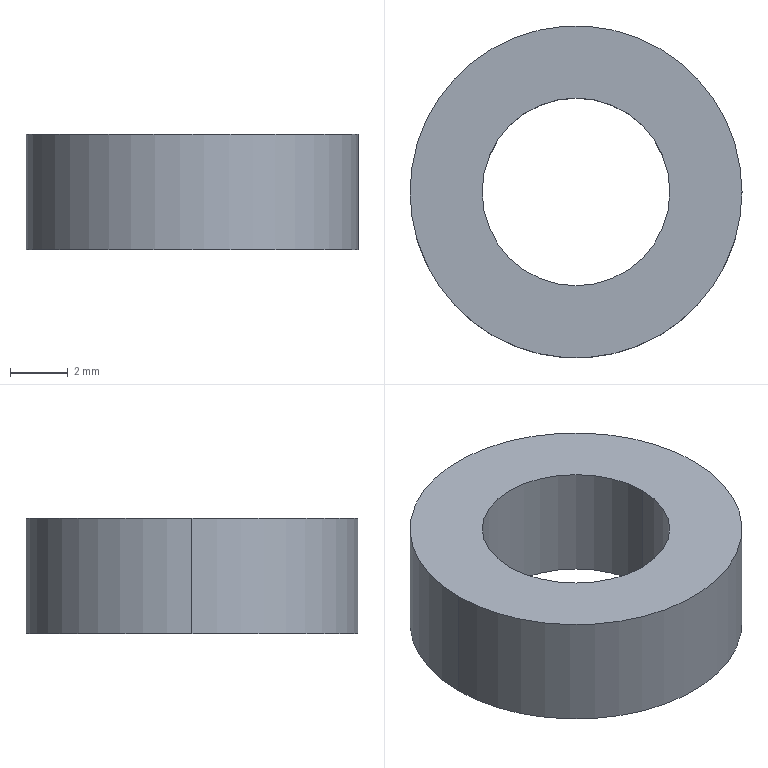Part | STEP file | Flip door spacer 001 | 1 solid | 6 faces | box 11.5 x 11.5 x 4 mm | volume 282.743 mm3 | cylinder 4 | plane 2 | commonest cylinder face diameters 6.5 x2 11.5 x2
STEP:
#1=CARTESIAN_POINT('',(0.,0.,0.));
#2=DIRECTION('',(0.,0.,1.));
#3=DIRECTION('',(1.,0.,0.));
#4=AXIS2_PLACEMENT_3D('',#1,#2,#3);
#5=CARTESIAN_POINT('',(-3.25,0.,4.));
#6=VERTEX_POINT('',#5);
#7=CARTESIAN_POINT('',(-3.25,0.,0.));
#8=VERTEX_POINT('',#7);
#9=CARTESIAN_POINT('',(-3.25,0.,4.));
#10=DIRECTION('',(0.,0.,-1.));
#11=VECTOR('',#10,1.);
#12=LINE('',#9,#11);
#13=CARTESIAN_POINT('',(0.,0.,4.));
#14=DIRECTION('',(0.,0.,-1.));
#15=DIRECTION('',(-1.,0.,0.));
#16=AXIS2_PLACEMENT_3D('',#13,#14,#15);
#17=CYLINDRICAL_SURFACE('',#16,3.25);
#18=CARTESIAN_POINT('',(6.283,0.));
#19=DIRECTION('',(0.,1.));
#20=VECTOR('',#19,1.);
#21=LINE('',#18,#20);
#22=(GEOMETRIC_REPRESENTATION_CONTEXT(2)PARAMETRIC_REPRESENTATION_CONTEXT()REPRESENTATION_CONTEXT('',''));
#23=DEFINITIONAL_REPRESENTATION('',(#21),#22);
#24=PCURVE('',#17,#23);
#25=CARTESIAN_POINT('',(0.,0.,4.));
#26=DIRECTION('',(0.,0.,-1.));
#27=DIRECTION('',(-1.,0.,0.));
#28=AXIS2_PLACEMENT_3D('',#25,#26,#27);
#29=CYLINDRICAL_SURFACE('',#28,3.25);
#30=CARTESIAN_POINT('',(0.,0.));
#31=DIRECTION('',(0.,1.));
#32=VECTOR('',#31,1.);
#33=LINE('',#30,#32);
#34=(GEOMETRIC_REPRESENTATION_CONTEXT(2)PARAMETRIC_REPRESENTATION_CONTEXT()REPRESENTATION_CONTEXT('',''));
#35=DEFINITIONAL_REPRESENTATION('',(#33),#34);
#36=PCURVE('',#29,#35);
#37=SURFACE_CURVE('',#12,(#24,#36),.PCURVE_S1.);
#38=EDGE_CURVE('',#6,#8,#37,.T.);
#39=ORIENTED_EDGE('',*,*,#38,.T.);
#40=CARTESIAN_POINT('',(3.25,0.,0.));
#41=VERTEX_POINT('',#40);
#42=CARTESIAN_POINT('',(0.,0.,0.));
#43=DIRECTION('',(0.,0.,1.));
#44=DIRECTION('',(1.,0.,0.));
#45=AXIS2_PLACEMENT_3D('',#42,#43,#44);
#46=CIRCLE('',#45,3.25);
#47=CARTESIAN_POINT('',(9.425,4.));
#48=DIRECTION('',(-1.,0.));
#49=VECTOR('',#48,1.);
#50=LINE('',#47,#49);
#51=(GEOMETRIC_REPRESENTATION_CONTEXT(2)PARAMETRIC_REPRESENTATION_CONTEXT()REPRESENTATION_CONTEXT('',''));
#52=DEFINITIONAL_REPRESENTATION('',(#50),#51);
#53=PCURVE('',#17,#52);
#54=CARTESIAN_POINT('',(0.,0.,0.));
#55=DIRECTION('',(0.,0.,1.));
#56=DIRECTION('',(1.,0.,0.));
#57=AXIS2_PLACEMENT_3D('',#54,#55,#56);
#58=PLANE('',#57);
#59=CARTESIAN_POINT('',(0.,0.));
#60=DIRECTION('',(1.,0.));
#61=AXIS2_PLACEMENT_2D('',#59,#60);
#62=CIRCLE('',#61,3.25);
#63=(GEOMETRIC_REPRESENTATION_CONTEXT(2)PARAMETRIC_REPRESENTATION_CONTEXT()REPRESENTATION_CONTEXT('',''));
#64=DEFINITIONAL_REPRESENTATION('',(#62),#63);
#65=PCURVE('',#58,#64);
#66=SURFACE_CURVE('',#46,(#53,#65),.PCURVE_S1.);
#67=EDGE_CURVE('',#8,#41,#66,.T.);
#68=ORIENTED_EDGE('',*,*,#67,.T.);
#69=CARTESIAN_POINT('',(3.25,0.,4.));
#70=VERTEX_POINT('',#69);
#71=CARTESIAN_POINT('',(3.25,0.,4.));
#72=DIRECTION('',(0.,0.,-1.));
#73=VECTOR('',#72,1.);
#74=LINE('',#71,#73);
#75=CARTESIAN_POINT('',(3.142,0.));
#76=DIRECTION('',(0.,1.));
#77=VECTOR('',#76,1.);
#78=LINE('',#75,#77);
#79=(GEOMETRIC_REPRESENTATION_CONTEXT(2)PARAMETRIC_REPRESENTATION_CONTEXT()REPRESENTATION_CONTEXT('',''));
#80=DEFINITIONAL_REPRESENTATION('',(#78),#79);
#81=PCURVE('',#17,#80);
#82=CARTESIAN_POINT('',(3.142,0.));
#83=DIRECTION('',(0.,1.));
#84=VECTOR('',#83,1.);
#85=LINE('',#82,#84);
#86=(GEOMETRIC_REPRESENTATION_CONTEXT(2)PARAMETRIC_REPRESENTATION_CONTEXT()REPRESENTATION_CONTEXT('',''));
#87=DEFINITIONAL_REPRESENTATION('',(#85),#86);
#88=PCURVE('',#29,#87);
#89=SURFACE_CURVE('',#74,(#81,#88),.PCURVE_S1.);
#90=EDGE_CURVE('',#70,#41,#89,.T.);
#91=ORIENTED_EDGE('',*,*,#90,.F.);
#92=CARTESIAN_POINT('',(0.,0.,4.));
#93=DIRECTION('',(0.,0.,1.));
#94=DIRECTION('',(1.,0.,0.));
#95=AXIS2_PLACEMENT_3D('',#92,#93,#94);
#96=CIRCLE('',#95,3.25);
#97=CARTESIAN_POINT('',(9.425,0.));
#98=DIRECTION('',(-1.,0.));
#99=VECTOR('',#98,1.);
#100=LINE('',#97,#99);
#101=(GEOMETRIC_REPRESENTATION_CONTEXT(2)PARAMETRIC_REPRESENTATION_CONTEXT()REPRESENTATION_CONTEXT('',''));
#102=DEFINITIONAL_REPRESENTATION('',(#100),#101);
#103=PCURVE('',#17,#102);
#104=CARTESIAN_POINT('',(0.,0.,4.));
#105=DIRECTION('',(0.,0.,1.));
#106=DIRECTION('',(1.,0.,0.));
#107=AXIS2_PLACEMENT_3D('',#104,#105,#106);
#108=PLANE('',#107);
#109=CARTESIAN_POINT('',(0.,0.));
#110=DIRECTION('',(1.,0.));
#111=AXIS2_PLACEMENT_2D('',#109,#110);
#112=CIRCLE('',#111,3.25);
#113=(GEOMETRIC_REPRESENTATION_CONTEXT(2)PARAMETRIC_REPRESENTATION_CONTEXT()REPRESENTATION_CONTEXT('',''));
#114=DEFINITIONAL_REPRESENTATION('',(#112),#113);
#115=PCURVE('',#108,#114);
#116=SURFACE_CURVE('',#96,(#103,#115),.PCURVE_S1.);
#117=EDGE_CURVE('',#6,#70,#116,.T.);
#118=ORIENTED_EDGE('',*,*,#117,.F.);
#119=EDGE_LOOP('',(#39,#68,#91,#118));
#120=FACE_BOUND('',#119,.F.);
#121=ADVANCED_FACE('',(#120),#17,.F.);
#122=CARTESIAN_POINT('',(5.75,0.,4.));
#123=VERTEX_POINT('',#122);
#124=CARTESIAN_POINT('',(-5.75,0.,4.));
#125=VERTEX_POINT('',#124);
#126=CARTESIAN_POINT('',(0.,0.,4.));
#127=DIRECTION('',(0.,0.,1.));
#128=DIRECTION('',(1.,0.,0.));
#129=AXIS2_PLACEMENT_3D('',#126,#127,#128);
#130=CIRCLE('',#129,5.75);
#131=CARTESIAN_POINT('',(0.,0.,4.));
#132=DIRECTION('',(0.,0.,-1.));
#133=DIRECTION('',(-1.,0.,0.));
#134=AXIS2_PLACEMENT_3D('',#131,#132,#133);
#135=CYLINDRICAL_SURFACE('',#134,5.75);
#136=CARTESIAN_POINT('',(3.142,0.));
#137=DIRECTION('',(-1.,0.));
#138=VECTOR('',#137,1.);
#139=LINE('',#136,#138);
#140=(GEOMETRIC_REPRESENTATION_CONTEXT(2)PARAMETRIC_REPRESENTATION_CONTEXT()REPRESENTATION_CONTEXT('',''));
#141=DEFINITIONAL_REPRESENTATION('',(#139),#140);
#142=PCURVE('',#135,#141);
#143=CARTESIAN_POINT('',(0.,0.));
#144=DIRECTION('',(1.,0.));
#145=AXIS2_PLACEMENT_2D('',#143,#144);
#146=CIRCLE('',#145,5.75);
#147=(GEOMETRIC_REPRESENTATION_CONTEXT(2)PARAMETRIC_REPRESENTATION_CONTEXT()REPRESENTATION_CONTEXT('',''));
#148=DEFINITIONAL_REPRESENTATION('',(#146),#147);
#149=PCURVE('',#108,#148);
#150=SURFACE_CURVE('',#130,(#142,#149),.PCURVE_S1.);
#151=EDGE_CURVE('',#123,#125,#150,.T.);
#152=ORIENTED_EDGE('',*,*,#151,.F.);
#153=CARTESIAN_POINT('',(5.75,0.,0.));
#154=VERTEX_POINT('',#153);
#155=CARTESIAN_POINT('',(5.75,0.,4.));
#156=DIRECTION('',(0.,0.,-1.));
#157=VECTOR('',#156,1.);
#158=LINE('',#155,#157);
#159=CARTESIAN_POINT('',(3.142,0.));
#160=DIRECTION('',(0.,1.));
#161=VECTOR('',#160,1.);
#162=LINE('',#159,#161);
#163=(GEOMETRIC_REPRESENTATION_CONTEXT(2)PARAMETRIC_REPRESENTATION_CONTEXT()REPRESENTATION_CONTEXT('',''));
#164=DEFINITIONAL_REPRESENTATION('',(#162),#163);
#165=PCURVE('',#135,#164);
#166=CARTESIAN_POINT('',(0.,0.,4.));
#167=DIRECTION('',(0.,0.,-1.));
#168=DIRECTION('',(-1.,0.,0.));
#169=AXIS2_PLACEMENT_3D('',#166,#167,#168);
#170=CYLINDRICAL_SURFACE('',#169,5.75);
#171=CARTESIAN_POINT('',(3.142,0.));
#172=DIRECTION('',(0.,1.));
#173=VECTOR('',#172,1.);
#174=LINE('',#171,#173);
#175=(GEOMETRIC_REPRESENTATION_CONTEXT(2)PARAMETRIC_REPRESENTATION_CONTEXT()REPRESENTATION_CONTEXT('',''));
#176=DEFINITIONAL_REPRESENTATION('',(#174),#175);
#177=PCURVE('',#170,#176);
#178=SURFACE_CURVE('',#158,(#165,#177),.PCURVE_S1.);
#179=EDGE_CURVE('',#123,#154,#178,.T.);
#180=ORIENTED_EDGE('',*,*,#179,.T.);
#181=CARTESIAN_POINT('',(-5.75,0.,0.));
#182=VERTEX_POINT('',#181);
#183=CARTESIAN_POINT('',(0.,0.,0.));
#184=DIRECTION('',(0.,0.,1.));
#185=DIRECTION('',(1.,0.,0.));
#186=AXIS2_PLACEMENT_3D('',#183,#184,#185);
#187=CIRCLE('',#186,5.75);
#188=CARTESIAN_POINT('',(3.142,4.));
#189=DIRECTION('',(-1.,0.));
#190=VECTOR('',#189,1.);
#191=LINE('',#188,#190);
#192=(GEOMETRIC_REPRESENTATION_CONTEXT(2)PARAMETRIC_REPRESENTATION_CONTEXT()REPRESENTATION_CONTEXT('',''));
#193=DEFINITIONAL_REPRESENTATION('',(#191),#192);
#194=PCURVE('',#135,#193);
#195=CARTESIAN_POINT('',(0.,0.));
#196=DIRECTION('',(1.,0.));
#197=AXIS2_PLACEMENT_2D('',#195,#196);
#198=CIRCLE('',#197,5.75);
#199=(GEOMETRIC_REPRESENTATION_CONTEXT(2)PARAMETRIC_REPRESENTATION_CONTEXT()REPRESENTATION_CONTEXT('',''));
#200=DEFINITIONAL_REPRESENTATION('',(#198),#199);
#201=PCURVE('',#58,#200);
#202=SURFACE_CURVE('',#187,(#194,#201),.PCURVE_S1.);
#203=EDGE_CURVE('',#154,#182,#202,.T.);
#204=ORIENTED_EDGE('',*,*,#203,.T.);
#205=CARTESIAN_POINT('',(-5.75,0.,4.));
#206=DIRECTION('',(0.,0.,-1.));
#207=VECTOR('',#206,1.);
#208=LINE('',#205,#207);
#209=CARTESIAN_POINT('',(0.,0.));
#210=DIRECTION('',(0.,1.));
#211=VECTOR('',#210,1.);
#212=LINE('',#209,#211);
#213=(GEOMETRIC_REPRESENTATION_CONTEXT(2)PARAMETRIC_REPRESENTATION_CONTEXT()REPRESENTATION_CONTEXT('',''));
#214=DEFINITIONAL_REPRESENTATION('',(#212),#213);
#215=PCURVE('',#135,#214);
#216=CARTESIAN_POINT('',(6.283,0.));
#217=DIRECTION('',(0.,1.));
#218=VECTOR('',#217,1.);
#219=LINE('',#216,#218);
#220=(GEOMETRIC_REPRESENTATION_CONTEXT(2)PARAMETRIC_REPRESENTATION_CONTEXT()REPRESENTATION_CONTEXT('',''));
#221=DEFINITIONAL_REPRESENTATION('',(#219),#220);
#222=PCURVE('',#170,#221);
#223=SURFACE_CURVE('',#208,(#215,#222),.PCURVE_S1.);
#224=EDGE_CURVE('',#125,#182,#223,.T.);
#225=ORIENTED_EDGE('',*,*,#224,.F.);
#226=EDGE_LOOP('',(#152,#180,#204,#225));
#227=FACE_BOUND('',#226,.T.);
#228=ADVANCED_FACE('',(#227),#135,.T.);
#229=CARTESIAN_POINT('',(0.,0.,4.));
#230=DIRECTION('',(0.,0.,1.));
#231=DIRECTION('',(1.,0.,0.));
#232=AXIS2_PLACEMENT_3D('',#229,#230,#231);
#233=CIRCLE('',#232,5.75);
#234=CARTESIAN_POINT('',(0.,0.));
#235=DIRECTION('',(1.,0.));
#236=AXIS2_PLACEMENT_2D('',#234,#235);
#237=CIRCLE('',#236,5.75);
#238=(GEOMETRIC_REPRESENTATION_CONTEXT(2)PARAMETRIC_REPRESENTATION_CONTEXT()REPRESENTATION_CONTEXT('',''));
#239=DEFINITIONAL_REPRESENTATION('',(#237),#238);
#240=PCURVE('',#108,#239);
#241=CARTESIAN_POINT('',(9.425,0.));
#242=DIRECTION('',(-1.,0.));
#243=VECTOR('',#242,1.);
#244=LINE('',#241,#243);
#245=(GEOMETRIC_REPRESENTATION_CONTEXT(2)PARAMETRIC_REPRESENTATION_CONTEXT()REPRESENTATION_CONTEXT('',''));
#246=DEFINITIONAL_REPRESENTATION('',(#244),#245);
#247=PCURVE('',#170,#246);
#248=SURFACE_CURVE('',#233,(#240,#247),.PCURVE_S1.);
#249=EDGE_CURVE('',#125,#123,#248,.T.);
#250=ORIENTED_EDGE('',*,*,#249,.T.);
#251=ORIENTED_EDGE('',*,*,#151,.T.);
#252=EDGE_LOOP('',(#250,#251));
#253=FACE_BOUND('',#252,.T.);
#254=ORIENTED_EDGE('',*,*,#117,.F.);
#255=CARTESIAN_POINT('',(0.,0.,4.));
#256=DIRECTION('',(0.,0.,1.));
#257=DIRECTION('',(1.,0.,0.));
#258=AXIS2_PLACEMENT_3D('',#255,#256,#257);
#259=CIRCLE('',#258,3.25);
#260=CARTESIAN_POINT('',(0.,0.));
#261=DIRECTION('',(1.,0.));
#262=AXIS2_PLACEMENT_2D('',#260,#261);
#263=CIRCLE('',#262,3.25);
#264=(GEOMETRIC_REPRESENTATION_CONTEXT(2)PARAMETRIC_REPRESENTATION_CONTEXT()REPRESENTATION_CONTEXT('',''));
#265=DEFINITIONAL_REPRESENTATION('',(#263),#264);
#266=PCURVE('',#108,#265);
#267=CARTESIAN_POINT('',(3.142,0.));
#268=DIRECTION('',(-1.,0.));
#269=VECTOR('',#268,1.);
#270=LINE('',#267,#269);
#271=(GEOMETRIC_REPRESENTATION_CONTEXT(2)PARAMETRIC_REPRESENTATION_CONTEXT()REPRESENTATION_CONTEXT('',''));
#272=DEFINITIONAL_REPRESENTATION('',(#270),#271);
#273=PCURVE('',#29,#272);
#274=SURFACE_CURVE('',#259,(#266,#273),.PCURVE_S1.);
#275=EDGE_CURVE('',#70,#6,#274,.T.);
#276=ORIENTED_EDGE('',*,*,#275,.F.);
#277=EDGE_LOOP('',(#254,#276));
#278=FACE_BOUND('',#277,.T.);
#279=ADVANCED_FACE('',(#253,#278),#108,.T.);
#280=CARTESIAN_POINT('',(0.,0.,0.));
#281=DIRECTION('',(0.,0.,1.));
#282=DIRECTION('',(1.,0.,0.));
#283=AXIS2_PLACEMENT_3D('',#280,#281,#282);
#284=CIRCLE('',#283,5.75);
#285=CARTESIAN_POINT('',(0.,0.));
#286=DIRECTION('',(1.,0.));
#287=AXIS2_PLACEMENT_2D('',#285,#286);
#288=CIRCLE('',#287,5.75);
#289=(GEOMETRIC_REPRESENTATION_CONTEXT(2)PARAMETRIC_REPRESENTATION_CONTEXT()REPRESENTATION_CONTEXT('',''));
#290=DEFINITIONAL_REPRESENTATION('',(#288),#289);
#291=PCURVE('',#58,#290);
#292=CARTESIAN_POINT('',(9.425,4.));
#293=DIRECTION('',(-1.,0.));
#294=VECTOR('',#293,1.);
#295=LINE('',#292,#294);
#296=(GEOMETRIC_REPRESENTATION_CONTEXT(2)PARAMETRIC_REPRESENTATION_CONTEXT()REPRESENTATION_CONTEXT('',''));
#297=DEFINITIONAL_REPRESENTATION('',(#295),#296);
#298=PCURVE('',#170,#297);
#299=SURFACE_CURVE('',#284,(#291,#298),.PCURVE_S1.);
#300=EDGE_CURVE('',#182,#154,#299,.T.);
#301=ORIENTED_EDGE('',*,*,#300,.F.);
#302=ORIENTED_EDGE('',*,*,#203,.F.);
#303=EDGE_LOOP('',(#301,#302));
#304=FACE_BOUND('',#303,.T.);
#305=ORIENTED_EDGE('',*,*,#67,.T.);
#306=CARTESIAN_POINT('',(0.,0.,0.));
#307=DIRECTION('',(0.,0.,1.));
#308=DIRECTION('',(1.,0.,0.));
#309=AXIS2_PLACEMENT_3D('',#306,#307,#308);
#310=CIRCLE('',#309,3.25);
#311=CARTESIAN_POINT('',(0.,0.));
#312=DIRECTION('',(1.,0.));
#313=AXIS2_PLACEMENT_2D('',#311,#312);
#314=CIRCLE('',#313,3.25);
#315=(GEOMETRIC_REPRESENTATION_CONTEXT(2)PARAMETRIC_REPRESENTATION_CONTEXT()REPRESENTATION_CONTEXT('',''));
#316=DEFINITIONAL_REPRESENTATION('',(#314),#315);
#317=PCURVE('',#58,#316);
#318=CARTESIAN_POINT('',(3.142,4.));
#319=DIRECTION('',(-1.,0.));
#320=VECTOR('',#319,1.);
#321=LINE('',#318,#320);
#322=(GEOMETRIC_REPRESENTATION_CONTEXT(2)PARAMETRIC_REPRESENTATION_CONTEXT()REPRESENTATION_CONTEXT('',''));
#323=DEFINITIONAL_REPRESENTATION('',(#321),#322);
#324=PCURVE('',#29,#323);
#325=SURFACE_CURVE('',#310,(#317,#324),.PCURVE_S1.);
#326=EDGE_CURVE('',#41,#8,#325,.T.);
#327=ORIENTED_EDGE('',*,*,#326,.T.);
#328=EDGE_LOOP('',(#305,#327));
#329=FACE_BOUND('',#328,.T.);
#330=ADVANCED_FACE('',(#304,#329),#58,.F.);
#331=ORIENTED_EDGE('',*,*,#179,.F.);
#332=ORIENTED_EDGE('',*,*,#249,.F.);
#333=ORIENTED_EDGE('',*,*,#224,.T.);
#334=ORIENTED_EDGE('',*,*,#300,.T.);
#335=EDGE_LOOP('',(#331,#332,#333,#334));
#336=FACE_BOUND('',#335,.T.);
#337=ADVANCED_FACE('',(#336),#170,.T.);
#338=ORIENTED_EDGE('',*,*,#326,.T.);
#339=ORIENTED_EDGE('',*,*,#38,.F.);
#340=ORIENTED_EDGE('',*,*,#275,.F.);
#341=ORIENTED_EDGE('',*,*,#90,.T.);
#342=EDGE_LOOP('',(#338,#339,#340,#341));
#343=FACE_BOUND('',#342,.F.);
#344=ADVANCED_FACE('',(#343),#29,.F.);
#345=CLOSED_SHELL('',(#121,#228,#279,#330,#337,#344));
#346=MANIFOLD_SOLID_BREP('',#345);
#347=(LENGTH_UNIT()NAMED_UNIT(*)SI_UNIT(.MILLI.,.METRE.));
#348=UNCERTAINTY_MEASURE_WITH_UNIT(LENGTH_MEASURE(0.0000001),#347,'','');
#349=(NAMED_UNIT(*)PLANE_ANGLE_UNIT()SI_UNIT($,.RADIAN.));
#350=(NAMED_UNIT(*)SI_UNIT($,.STERADIAN.)SOLID_ANGLE_UNIT());
#351=(GEOMETRIC_REPRESENTATION_CONTEXT(3)GLOBAL_UNCERTAINTY_ASSIGNED_CONTEXT((#348))GLOBAL_UNIT_ASSIGNED_CONTEXT((#347,#349,#350))REPRESENTATION_CONTEXT('',''));
#352=ADVANCED_BREP_SHAPE_REPRESENTATION('',(#4,#346),#351);